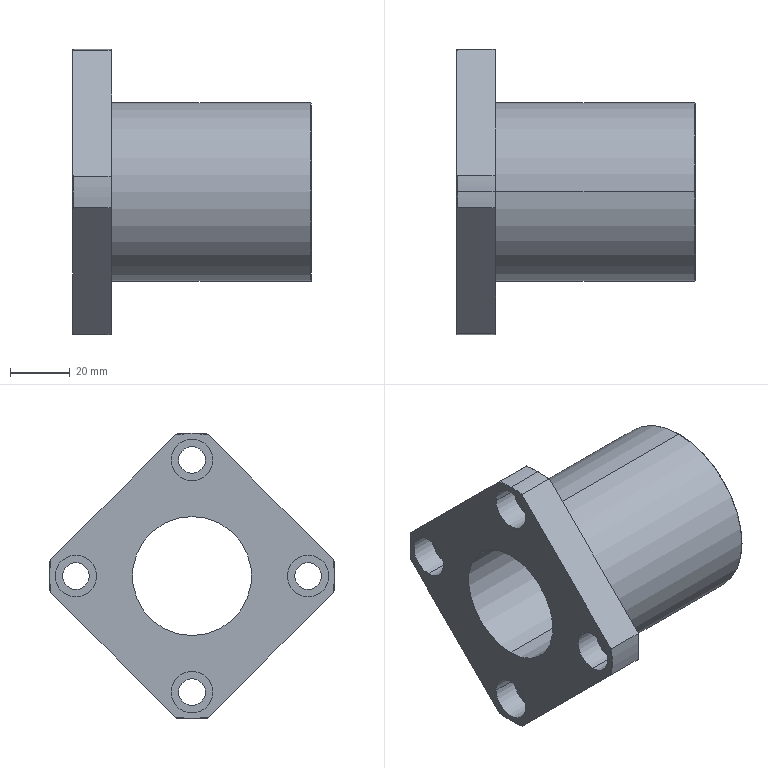Part | SolidWorks | features BaseBody 1 | 1 solid | 48 faces | box 80 x 96 x 96 mm | volume 154247 mm3 | cylinder 25 | torus 12 | plane 11 | commonest cylinder face diameters 9 x8 14 x8 96 x5 40 x2 60 x2